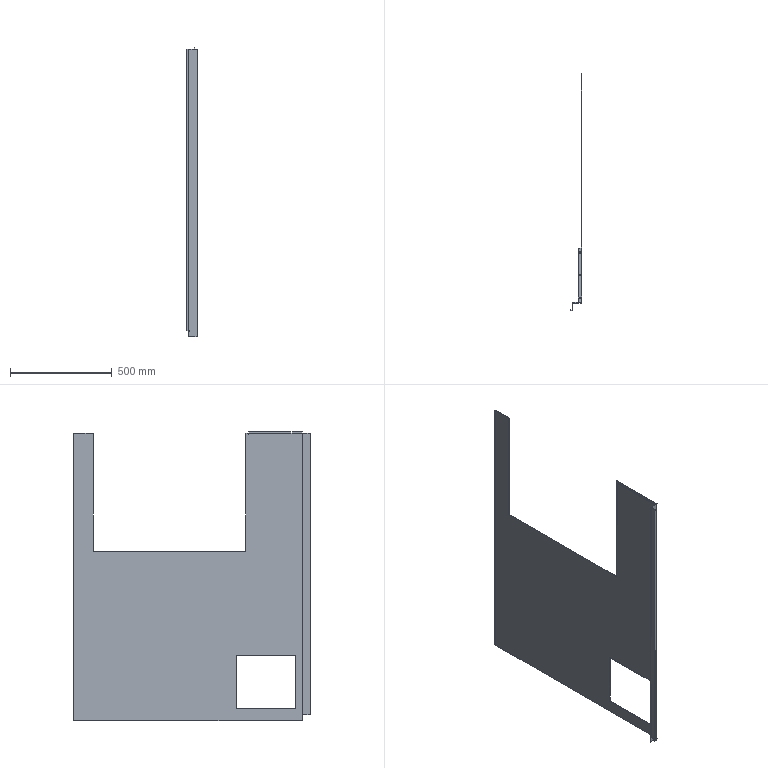Part | STEP file | Right Side Plate | 1 solid | 58 faces | box 55 x 1166 x 1423 mm | volume 2424332 mm3 | plane 39 | cylinder 19 | commonest cylinder face diameters 1 x8 7 x6 5 x5